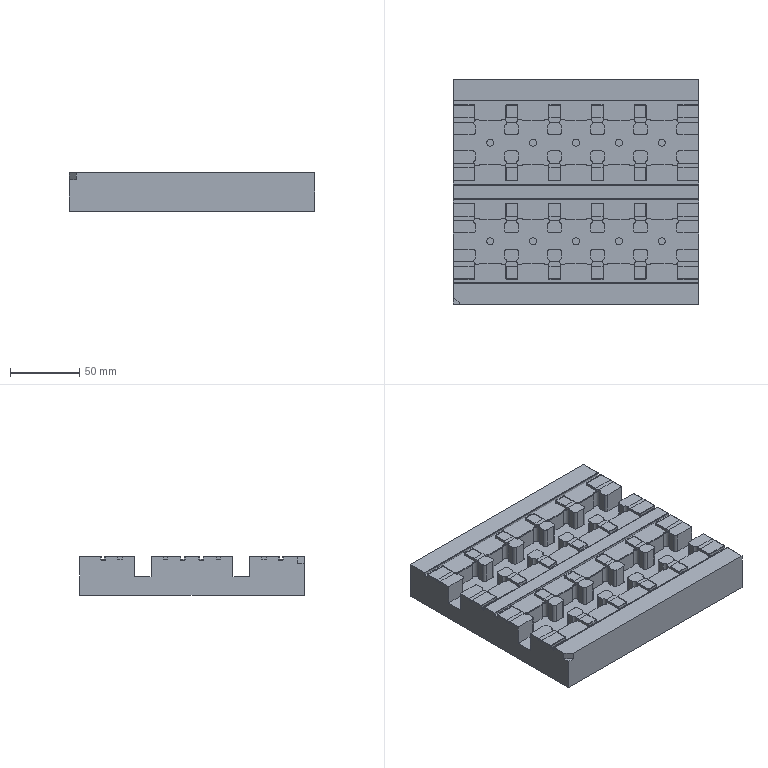NC program | NX | posted by the shop | part box 177 x 162 x 28 mm
Lines 1 to 616 of 254847:
%
O0001
(Machine time: 185.94 MIN)
(===Total Tool:12===)
(T2=D17R0.8FlyCutter D=17.  R=0.8  D-  H02 Z=28.1  )
(T17=C6SpotDrill  D=6.   R=0.   D-  H17 Z=12.7  )
(T15=ZT4.5  D=4.5  DR_a=118 D-  H15 Z=13.5  )
(T10=D10    D=10.  R=0.   D-  H10 Z=13.56 )
(T5=D4      D=4.   R=0.   D5  H05 Z=13.55 )
(T4=D3      D=3.   R=0.   D4  H04 Z=25.32 )
(T3=ZT5.1   D=5.1  DR_a=118 D-  H03 Z=1.35  )
(T11=D10-J  D=10.  R=0.   D-  H11 Z=28.   )
(T14=D4-J   D=4.   R=0.   D-  H14 Z=13.5  )
(T13=D3-J   D=3.   R=0.   D-  H13 Z=25.3  )
(T1=D6ChamferMill   D=6.   R=0.   D-  H01 Z=11.9  )
(T7=D6-J    D=6.   R=0.   D7  H07 Z=23.   )
G80 G90 G17 G49 G40
G91 G28 Z0
M01
N1 T02 M06
(D17R0.8FlyCutter  D=17. R=0.8 H=02 ce=0.20 di=0.10)
(MAX_Z=43. MIN_Z=28.1 Time=9.23M)
T17
G00 G90 G54 X109. Y-78.971 M03 S2000
G43 H02 Z43.
M08
Z31.9
G01 Z29.9 F2500.
X97.
X-95.301
G02 X-97. Y-77.272 I.001 J1.7
G01 Y-69.971
G02 X-95.47 Y-68.441 I1.53 J0.0
G01 X95.301
G03 X97. Y-66.742 I-.001 J1.7
G01 Y-59.612
G03 X95.3 Y-57.912 I-1.7 J0.0
G01 X-95.301
G02 X-97. Y-56.213 I.001 J1.7
G01 Y-49.082
G02 X-95.3 Y-47.382 I1.7 J0.0
G01 X95.301
G03 X97. Y-45.684 I-.001 J1.7
G01 Y-38.553
G03 X95.3 Y-36.853 I-1.7 J0.0
G01 X-95.301
G02 X-97. Y-35.154 I.001 J1.7
G01 Y-28.024
G02 X-95.3 Y-26.324 I1.7 J0.0
G01 X95.301
G03 X97. Y-24.625 I-.001 J1.7
G01 Y-17.494
G03 X95.3 Y-15.794 I-1.7 J0.0
G01 X-95.301
G02 X-97. Y-14.095 I.001 J1.7
G01 Y-6.965
G02 X-95.3 Y-5.265 I1.7 J0.0
G01 X95.301
G03 X97. Y-3.566 I-.001 J1.7
G01 Y3.565
G03 X95.3 Y5.265 I-1.7 J0.0
G01 X-95.301
G02 X-97. Y6.963 I.001 J1.7
G01 Y14.094
G02 X-95.3 Y15.794 I1.7 J0.0
G01 X95.301
G03 X97. Y17.493 I-.001 J1.7
G01 Y24.624
G03 X95.3 Y26.324 I-1.7 J0.0
G01 X-95.301
G02 X-97. Y28.022 I.001 J1.7
G01 Y35.153
G02 X-95.3 Y36.853 I1.7 J0.0
G01 X95.301
G03 X97. Y38.552 I-.001 J1.7
G01 Y45.682
G03 X95.3 Y47.382 I-1.7 J0.0
G01 X-95.301
G02 X-97. Y49.081 I.001 J1.7
G01 Y56.212
G02 X-95.3 Y57.912 I1.7 J0.0
G01 X95.301
G03 X97. Y59.611 I-.001 J1.7
G01 Y66.741
G03 X95.3 Y68.441 I-1.7 J0.0
G01 X-95.301
G02 X-97. Y70.14 I.001 J1.7
G01 Y77.271
G02 X-95.3 Y78.971 I1.7 J0.0
G01 X97.
X109.
Z31.9
G00 Z33.2
Y-78.971
Z31.6
G01 Z29.6
X97.
X-95.301
G02 X-97. Y-77.272 I.001 J1.7
G01 Y-69.971
G02 X-95.47 Y-68.441 I1.53 J0.0
G01 X95.301
G03 X97. Y-66.742 I-.001 J1.7
G01 Y-59.612
G03 X95.3 Y-57.912 I-1.7 J0.0
G01 X-95.301
G02 X-97. Y-56.213 I.001 J1.7
G01 Y-49.082
G02 X-95.3 Y-47.382 I1.7 J0.0
G01 X95.301
G03 X97. Y-45.684 I-.001 J1.7
G01 Y-38.553
G03 X95.3 Y-36.853 I-1.7 J0.0
G01 X-95.301
G02 X-97. Y-35.154 I.001 J1.7
G01 Y-28.024
G02 X-95.3 Y-26.324 I1.7 J0.0
G01 X95.301
G03 X97. Y-24.625 I-.001 J1.7
G01 Y-17.494
G03 X95.3 Y-15.794 I-1.7 J0.0
G01 X-95.301
G02 X-97. Y-14.095 I.001 J1.7
G01 Y-6.965
G02 X-95.3 Y-5.265 I1.7 J0.0
G01 X95.301
G03 X97. Y-3.566 I-.001 J1.7
G01 Y3.565
G03 X95.3 Y5.265 I-1.7 J0.0
G01 X-95.301
G02 X-97. Y6.963 I.001 J1.7
G01 Y14.094
G02 X-95.3 Y15.794 I1.7 J0.0
G01 X95.301
G03 X97. Y17.493 I-.001 J1.7
G01 Y24.624
G03 X95.3 Y26.324 I-1.7 J0.0
G01 X-95.301
G02 X-97. Y28.022 I.001 J1.7
G01 Y35.153
G02 X-95.3 Y36.853 I1.7 J0.0
G01 X95.301
G03 X97. Y38.552 I-.001 J1.7
G01 Y45.682
G03 X95.3 Y47.382 I-1.7 J0.0
G01 X-95.301
G02 X-97. Y49.081 I.001 J1.7
G01 Y56.212
G02 X-95.3 Y57.912 I1.7 J0.0
G01 X95.301
G03 X97. Y59.611 I-.001 J1.7
G01 Y66.741
G03 X95.3 Y68.441 I-1.7 J0.0
G01 X-95.301
G02 X-97. Y70.14 I.001 J1.7
G01 Y77.271
G02 X-95.3 Y78.971 I1.7 J0.0
G01 X97.
X109.
Z31.6
G00 Z32.9
Y-78.971
Z31.3
G01 Z29.3
X97.
X-95.301
G02 X-97. Y-77.272 I.001 J1.7
G01 Y-69.971
G02 X-95.47 Y-68.441 I1.53 J0.0
G01 X95.301
G03 X97. Y-66.742 I-.001 J1.7
G01 Y-59.612
G03 X95.3 Y-57.912 I-1.7 J0.0
G01 X-95.301
G02 X-97. Y-56.213 I.001 J1.7
G01 Y-49.082
G02 X-95.3 Y-47.382 I1.7 J0.0
G01 X95.301
G03 X97. Y-45.684 I-.001 J1.7
G01 Y-38.553
G03 X95.3 Y-36.853 I-1.7 J0.0
G01 X-95.301
G02 X-97. Y-35.154 I.001 J1.7
G01 Y-28.024
G02 X-95.3 Y-26.324 I1.7 J0.0
G01 X95.301
G03 X97. Y-24.625 I-.001 J1.7
G01 Y-17.494
G03 X95.3 Y-15.794 I-1.7 J0.0
G01 X-95.301
G02 X-97. Y-14.095 I.001 J1.7
G01 Y-6.965
G02 X-95.3 Y-5.265 I1.7 J0.0
G01 X95.301
G03 X97. Y-3.566 I-.001 J1.7
G01 Y3.565
G03 X95.3 Y5.265 I-1.7 J0.0
G01 X-95.301
G02 X-97. Y6.963 I.001 J1.7
G01 Y14.094
G02 X-95.3 Y15.794 I1.7 J0.0
G01 X95.301
G03 X97. Y17.493 I-.001 J1.7
G01 Y24.624
G03 X95.3 Y26.324 I-1.7 J0.0
G01 X-95.301
G02 X-97. Y28.022 I.001 J1.7
G01 Y35.153
G02 X-95.3 Y36.853 I1.7 J0.0
G01 X95.301
G03 X97. Y38.552 I-.001 J1.7
G01 Y45.682
G03 X95.3 Y47.382 I-1.7 J0.0
G01 X-95.301
G02 X-97. Y49.081 I.001 J1.7
G01 Y56.212
G02 X-95.3 Y57.912 I1.7 J0.0
G01 X95.301
G03 X97. Y59.611 I-.001 J1.7
G01 Y66.741
G03 X95.3 Y68.441 I-1.7 J0.0
G01 X-95.301
G02 X-97. Y70.14 I.001 J1.7
G01 Y77.271
G02 X-95.3 Y78.971 I1.7 J0.0
G01 X97.
X109.
Z31.3
G00 Z32.6
Y-78.971
Z31.
G01 Z29.
X97.
X-95.301
G02 X-97. Y-77.272 I.001 J1.7
G01 Y-69.971
G02 X-95.47 Y-68.441 I1.53 J0.0
G01 X95.301
G03 X97. Y-66.742 I-.001 J1.7
G01 Y-59.612
G03 X95.3 Y-57.912 I-1.7 J0.0
G01 X-95.301
G02 X-97. Y-56.213 I.001 J1.7
G01 Y-49.082
G02 X-95.3 Y-47.382 I1.7 J0.0
G01 X95.301
G03 X97. Y-45.684 I-.001 J1.7
G01 Y-38.553
G03 X95.3 Y-36.853 I-1.7 J0.0
G01 X-95.301
G02 X-97. Y-35.154 I.001 J1.7
G01 Y-28.024
G02 X-95.3 Y-26.324 I1.7 J0.0
G01 X95.301
G03 X97. Y-24.625 I-.001 J1.7
G01 Y-17.494
G03 X95.3 Y-15.794 I-1.7 J0.0
G01 X-95.301
G02 X-97. Y-14.095 I.001 J1.7
G01 Y-6.965
G02 X-95.3 Y-5.265 I1.7 J0.0
G01 X95.301
G03 X97. Y-3.566 I-.001 J1.7
G01 Y3.565
G03 X95.3 Y5.265 I-1.7 J0.0
G01 X-95.301
G02 X-97. Y6.963 I.001 J1.7
G01 Y14.094
G02 X-95.3 Y15.794 I1.7 J0.0
G01 X95.301
G03 X97. Y17.493 I-.001 J1.7
G01 Y24.624
G03 X95.3 Y26.324 I-1.7 J0.0
G01 X-95.301
G02 X-97. Y28.022 I.001 J1.7
G01 Y35.153
G02 X-95.3 Y36.853 I1.7 J0.0
G01 X95.301
G03 X97. Y38.552 I-.001 J1.7
G01 Y45.682
G03 X95.3 Y47.382 I-1.7 J0.0
G01 X-95.301
G02 X-97. Y49.081 I.001 J1.7
G01 Y56.212
G02 X-95.3 Y57.912 I1.7 J0.0
G01 X95.301
G03 X97. Y59.611 I-.001 J1.7
G01 Y66.741
G03 X95.3 Y68.441 I-1.7 J0.0
G01 X-95.301
G02 X-97. Y70.14 I.001 J1.7
G01 Y77.271
G02 X-95.3 Y78.971 I1.7 J0.0
G01 X97.
X109.
Z31.
G00 Z32.3
Y-78.971
Z30.7
G01 Z28.7
X97.
X-95.301
G02 X-97. Y-77.272 I.001 J1.7
G01 Y-69.971
G02 X-95.47 Y-68.441 I1.53 J0.0
G01 X95.301
G03 X97. Y-66.742 I-.001 J1.7
G01 Y-59.612
G03 X95.3 Y-57.912 I-1.7 J0.0
G01 X-95.301
G02 X-97. Y-56.213 I.001 J1.7
G01 Y-49.082
G02 X-95.3 Y-47.382 I1.7 J0.0
G01 X95.301
G03 X97. Y-45.684 I-.001 J1.7
G01 Y-38.553
G03 X95.3 Y-36.853 I-1.7 J0.0
G01 X-95.301
G02 X-97. Y-35.154 I.001 J1.7
G01 Y-28.024
G02 X-95.3 Y-26.324 I1.7 J0.0
G01 X95.301
G03 X97. Y-24.625 I-.001 J1.7
G01 Y-17.494
G03 X95.3 Y-15.794 I-1.7 J0.0
G01 X-95.301
G02 X-97. Y-14.095 I.001 J1.7
G01 Y-6.965
G02 X-95.3 Y-5.265 I1.7 J0.0
G01 X95.301
G03 X97. Y-3.566 I-.001 J1.7
G01 Y3.565
G03 X95.3 Y5.265 I-1.7 J0.0
G01 X-95.301
G02 X-97. Y6.963 I.001 J1.7
G01 Y14.094
G02 X-95.3 Y15.794 I1.7 J0.0
G01 X95.301
G03 X97. Y17.493 I-.001 J1.7
G01 Y24.624
G03 X95.3 Y26.324 I-1.7 J0.0
G01 X-95.301
G02 X-97. Y28.022 I.001 J1.7
G01 Y35.153
G02 X-95.3 Y36.853 I1.7 J0.0
G01 X95.301
G03 X97. Y38.552 I-.001 J1.7
G01 Y45.682
G03 X95.3 Y47.382 I-1.7 J0.0
G01 X-95.301
G02 X-97. Y49.081 I.001 J1.7
G01 Y56.212
G02 X-95.3 Y57.912 I1.7 J0.0
G01 X95.301
G03 X97. Y59.611 I-.001 J1.7
G01 Y66.741
G03 X95.3 Y68.441 I-1.7 J0.0
G01 X-95.301
G02 X-97. Y70.14 I.001 J1.7
G01 Y77.271
G02 X-95.3 Y78.971 I1.7 J0.0
G01 X97.
X109.
Z30.7
G00 Z32.
Y-78.971
Z30.4
G01 Z28.4
X97.
X-95.301
G02 X-97. Y-77.272 I.001 J1.7
G01 Y-69.971
G02 X-95.47 Y-68.441 I1.53 J0.0
G01 X95.301
G03 X97. Y-66.742 I-.001 J1.7
G01 Y-59.612
G03 X95.3 Y-57.912 I-1.7 J0.0
G01 X-95.301
G02 X-97. Y-56.213 I.001 J1.7
G01 Y-49.082
G02 X-95.3 Y-47.382 I1.7 J0.0
G01 X95.301
G03 X97. Y-45.684 I-.001 J1.7
G01 Y-38.553
G03 X95.3 Y-36.853 I-1.7 J0.0
G01 X-95.301
G02 X-97. Y-35.154 I.001 J1.7
G01 Y-28.024
G02 X-95.3 Y-26.324 I1.7 J0.0
G01 X95.301
G03 X97. Y-24.625 I-.001 J1.7
G01 Y-17.494
G03 X95.3 Y-15.794 I-1.7 J0.0
G01 X-95.301
G02 X-97. Y-14.095 I.001 J1.7
G01 Y-6.965
G02 X-95.3 Y-5.265 I1.7 J0.0
G01 X95.301
G03 X97. Y-3.566 I-.001 J1.7
G01 Y3.565
G03 X95.3 Y5.265 I-1.7 J0.0
G01 X-95.301
G02 X-97. Y6.963 I.001 J1.7
G01 Y14.094
G02 X-95.3 Y15.794 I1.7 J0.0
G01 X95.301
G03 X97. Y17.493 I-.001 J1.7
G01 Y24.624
G03 X95.3 Y26.324 I-1.7 J0.0
G01 X-95.301
G02 X-97. Y28.022 I.001 J1.7
G01 Y35.153
G02 X-95.3 Y36.853 I1.7 J0.0
G01 X95.301
G03 X97. Y38.552 I-.001 J1.7
G01 Y45.682
G03 X95.3 Y47.382 I-1.7 J0.0
G01 X-95.301
G02 X-97. Y49.081 I.001 J1.7
G01 Y56.212
G02 X-95.3 Y57.912 I1.7 J0.0
G01 X95.301
G03 X97. Y59.611 I-.001 J1.7
G01 Y66.741
G03 X95.3 Y68.441 I-1.7 J0.0
G01 X-95.301
G02 X-97. Y70.14 I.001 J1.7
G01 Y77.271
G02 X-95.3 Y78.971 I1.7 J0.0
G01 X97.
X109.
Z30.4
G00 Z31.7
Y-78.971
Z30.1
G01 Z28.1
X97.
X-95.301
G02 X-97. Y-77.272 I.001 J1.7
G01 Y-69.971
G02 X-95.47 Y-68.441 I1.53 J0.0
G01 X95.301
G03 X97. Y-66.742 I-.001 J1.7
G01 Y-59.612
G03 X95.3 Y-57.912 I-1.7 J0.0
G01 X-95.301
G02 X-97. Y-56.213 I.001 J1.7
G01 Y-49.082
G02 X-95.3 Y-47.382 I1.7 J0.0
G01 X95.301
G03 X97. Y-45.684 I-.001 J1.7
G01 Y-38.553
G03 X95.3 Y-36.853 I-1.7 J0.0
G01 X-95.301
G02 X-97. Y-35.154 I.001 J1.7
G01 Y-28.024
G02 X-95.3 Y-26.324 I1.7 J0.0
G01 X95.301
G03 X97. Y-24.625 I-.001 J1.7
G01 Y-17.494
G03 X95.3 Y-15.794 I-1.7 J0.0
G01 X-95.301
G02 X-97. Y-14.095 I.001 J1.7
G01 Y-6.965
G02 X-95.3 Y-5.265 I1.7 J0.0
G01 X95.301
G03 X97. Y-3.566 I-.001 J1.7
G01 Y3.565
G03 X95.3 Y5.265 I-1.7 J0.0
G01 X-95.301
G02 X-97. Y6.963 I.001 J1.7
G01 Y14.094
G02 X-95.3 Y15.794 I1.7 J0.0
G01 X95.301
G03 X97. Y17.493 I-.001 J1.7
G01 Y24.624
G03 X95.3 Y26.324 I-1.7 J0.0
G01 X-95.301
G02 X-97. Y28.022 I.001 J1.7
G01 Y35.153
G02 X-95.3 Y36.853 I1.7 J0.0
G01 X95.301
G03 X97. Y38.552 I-.001 J1.7
G01 Y45.682
G03 X95.3 Y47.382 I-1.7 J0.0
G01 X-95.301
G02 X-97. Y49.081 I.001 J1.7
G01 Y56.212
G02 X-95.3 Y57.912 I1.7 J0.0
G01 X95.301
G03 X97. Y59.611 I-.001 J1.7
G01 Y66.741
G03 X95.3 Y68.441 I-1.7 J0.0
G01 X-95.301
G02 X-97. Y70.14 I.001 J1.7
G01 Y77.271
G02 X-95.3 Y78.971 I1.7 J0.0
G01 X97.
X109.
Z30.1
G00 Z43.
G91 G28 Z0.0
M05
M09
G91 G28 Z0.0
M01
N2 T17 M06
(C6SpotDrill  D=6. R=0. H=17 ce=0.00 di=0.10)
(MAX_Z=43. MIN_Z=27.2 Time=1.50M)
T15
G00 G90 G54 X-71.477 Y50.097 M03 S1500
G43 H17 Z43.
M08
G98 G81 X-71.477 Y50.097 Z27.2 R29. F50.
X-52.523
X-40.477
X-21.523
X-9.477
X9.477
X21.523
X40.477
X52.523
X71.477
Y21.103
X52.523
X40.477
X21.523
X9.477
X-9.477
X-21.523
X-40.477
X-52.523
X-71.477
Y-21.103
X-52.523
X-40.477
X-21.523
X-9.477
X9.477
X21.523
X40.477
X52.523
X71.477
Y-50.097
X52.523
X40.477
X21.523
X9.477
X-9.477
X-21.523
X-40.477
X-52.523
X-71.477
G80
G00 Z43.
G91 G28 Z0.0
M05
M09
G91 G28 Z0.0
M01
N3 T15 M06
(ZT4.5 D=4.5 DR_a=118 H=15)
(MAX_Z=43. MIN_Z=13.5 Time=12.46M)
T10
G00 G90 G54 X-71.477 Y50.097 M03 S1500
G43 H15 Z43.
M08
G98 G83 X-71.477 Y50.097 Z13.5 R29. F50. Q1.
X-52.523
X-40.477
X-21.523
X-9.477
X9.477
X21.523
X40.477
X52.523
X71.477
Y21.103
X52.523
X40.477
X21.523
X9.477
X-9.477
X-21.523
X-40.477
X-52.523
X-71.477
Y-21.103
X-52.523
X-40.477
X-21.523
X-9.477
X9.477
X21.523
X40.477
X52.523
X71.477
Y-50.097
X52.523
X40.477
X21.523
X9.477
X-9.477
X-21.523
X-40.477
X-52.523
X-71.477
G80
G00 Z43.
G91 G28 Z0.0
M05
M09
G91 G28 Z0.0
M01